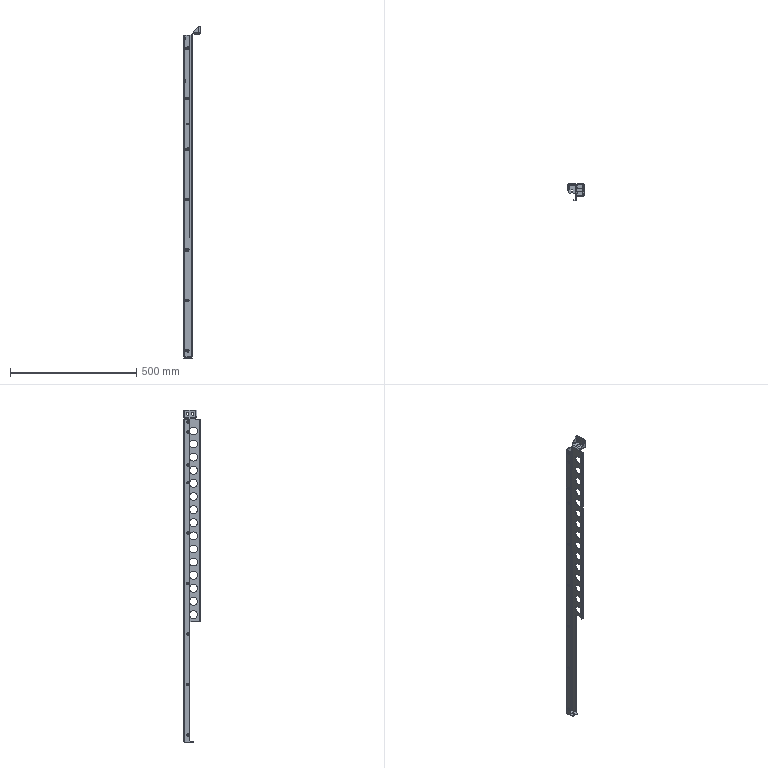Part | STEP file | 64560387 | 1 solid | 287 faces | box 64 x 67 x 1316 mm | volume 321357 mm3 | cylinder 121 | plane 102 | torus 64 | commonest cylinder face diameters 3.3 x32 8.3 x32 31 x30 5 x6 10 x6 7 x5